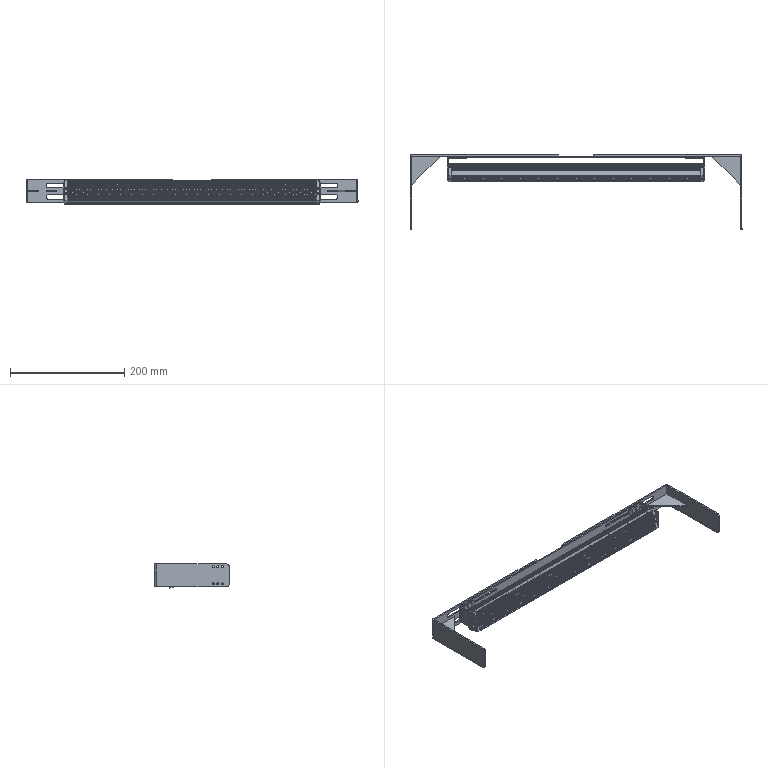Part | SolidWorks | 26 solids | 3161 faces | volume 230759 mm3 | spline 1080 | cylinder 934 | plane 897 | cone 250 | commonest cylinder face diameters 2 x434 1.9 x216 0.2 x90 3.3 x64 0.6 x24 4 x24